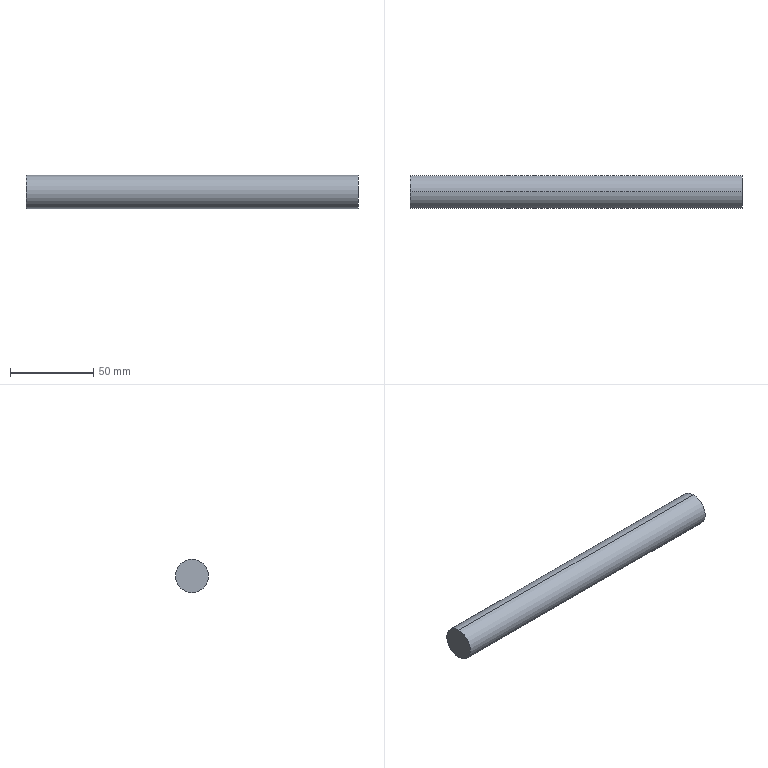Part | STEP file | B1-009 | 1 solid | 8 faces | box 200 x 20 x 20 mm | volume 62632 mm3 | cylinder 4 | cone 2 | plane 2 | commonest cylinder face diameters 4.2 x2 20 x2
STEP:
#1=CARTESIAN_POINT('',(0.,0.,0.));
#2=DIRECTION('',(0.,0.,1.));
#3=DIRECTION('',(1.,0.,0.));
#4=AXIS2_PLACEMENT_3D('',#1,#2,#3);
#5=CARTESIAN_POINT('',(86.,0.,-2.1));
#6=VERTEX_POINT('',#5);
#7=CARTESIAN_POINT('',(100.,0.,-2.1));
#8=VERTEX_POINT('',#7);
#9=CARTESIAN_POINT('',(100.,0.,-2.1));
#10=DIRECTION('',(1.,0.,0.));
#11=VECTOR('',#10,1.);
#12=LINE('',#9,#11);
#13=CARTESIAN_POINT('',(100.,0.,0.));
#14=DIRECTION('',(1.,0.,0.));
#15=DIRECTION('',(0.,0.,-1.));
#16=AXIS2_PLACEMENT_3D('',#13,#14,#15);
#17=CYLINDRICAL_SURFACE('',#16,2.1);
#18=CARTESIAN_POINT('',(6.283,0.));
#19=DIRECTION('',(0.,1.));
#20=VECTOR('',#19,1.);
#21=LINE('',#18,#20);
#22=(GEOMETRIC_REPRESENTATION_CONTEXT(2)PARAMETRIC_REPRESENTATION_CONTEXT()REPRESENTATION_CONTEXT('',''));
#23=DEFINITIONAL_REPRESENTATION('',(#21),#22);
#24=PCURVE('',#17,#23);
#25=CARTESIAN_POINT('',(100.,0.,0.));
#26=DIRECTION('',(1.,0.,0.));
#27=DIRECTION('',(0.,0.,-1.));
#28=AXIS2_PLACEMENT_3D('',#25,#26,#27);
#29=CYLINDRICAL_SURFACE('',#28,2.1);
#30=CARTESIAN_POINT('',(0.,0.));
#31=DIRECTION('',(0.,1.));
#32=VECTOR('',#31,1.);
#33=LINE('',#30,#32);
#34=(GEOMETRIC_REPRESENTATION_CONTEXT(2)PARAMETRIC_REPRESENTATION_CONTEXT()REPRESENTATION_CONTEXT('',''));
#35=DEFINITIONAL_REPRESENTATION('',(#33),#34);
#36=PCURVE('',#29,#35);
#37=SURFACE_CURVE('',#12,(#24,#36),.PCURVE_S1.);
#38=EDGE_CURVE('',#6,#8,#37,.T.);
#39=ORIENTED_EDGE('',*,*,#38,.T.);
#40=CARTESIAN_POINT('',(100.,0.,2.1));
#41=VERTEX_POINT('',#40);
#42=CARTESIAN_POINT('',(100.,0.,0.));
#43=DIRECTION('',(1.,0.,0.));
#44=DIRECTION('',(0.,0.,-1.));
#45=AXIS2_PLACEMENT_3D('',#42,#43,#44);
#46=CIRCLE('',#45,2.1);
#47=CARTESIAN_POINT('',(0.,0.));
#48=DIRECTION('',(1.,0.));
#49=VECTOR('',#48,1.);
#50=LINE('',#47,#49);
#51=(GEOMETRIC_REPRESENTATION_CONTEXT(2)PARAMETRIC_REPRESENTATION_CONTEXT()REPRESENTATION_CONTEXT('',''));
#52=DEFINITIONAL_REPRESENTATION('',(#50),#51);
#53=PCURVE('',#17,#52);
#54=CARTESIAN_POINT('',(100.,0.,0.));
#55=DIRECTION('',(1.,0.,0.));
#56=DIRECTION('',(0.,0.,-1.));
#57=AXIS2_PLACEMENT_3D('',#54,#55,#56);
#58=PLANE('',#57);
#59=CARTESIAN_POINT('',(0.,0.));
#60=DIRECTION('',(1.,0.));
#61=AXIS2_PLACEMENT_2D('',#59,#60);
#62=CIRCLE('',#61,2.1);
#63=(GEOMETRIC_REPRESENTATION_CONTEXT(2)PARAMETRIC_REPRESENTATION_CONTEXT()REPRESENTATION_CONTEXT('',''));
#64=DEFINITIONAL_REPRESENTATION('',(#62),#63);
#65=PCURVE('',#58,#64);
#66=SURFACE_CURVE('',#46,(#53,#65),.PCURVE_S1.);
#67=EDGE_CURVE('',#41,#8,#66,.T.);
#68=ORIENTED_EDGE('',*,*,#67,.F.);
#69=CARTESIAN_POINT('',(86.,0.,2.1));
#70=VERTEX_POINT('',#69);
#71=CARTESIAN_POINT('',(100.,0.,2.1));
#72=DIRECTION('',(1.,0.,0.));
#73=VECTOR('',#72,1.);
#74=LINE('',#71,#73);
#75=CARTESIAN_POINT('',(3.142,0.));
#76=DIRECTION('',(0.,1.));
#77=VECTOR('',#76,1.);
#78=LINE('',#75,#77);
#79=(GEOMETRIC_REPRESENTATION_CONTEXT(2)PARAMETRIC_REPRESENTATION_CONTEXT()REPRESENTATION_CONTEXT('',''));
#80=DEFINITIONAL_REPRESENTATION('',(#78),#79);
#81=PCURVE('',#17,#80);
#82=CARTESIAN_POINT('',(3.142,0.));
#83=DIRECTION('',(0.,1.));
#84=VECTOR('',#83,1.);
#85=LINE('',#82,#84);
#86=(GEOMETRIC_REPRESENTATION_CONTEXT(2)PARAMETRIC_REPRESENTATION_CONTEXT()REPRESENTATION_CONTEXT('',''));
#87=DEFINITIONAL_REPRESENTATION('',(#85),#86);
#88=PCURVE('',#29,#87);
#89=SURFACE_CURVE('',#74,(#81,#88),.PCURVE_S1.);
#90=EDGE_CURVE('',#70,#41,#89,.T.);
#91=ORIENTED_EDGE('',*,*,#90,.F.);
#92=CARTESIAN_POINT('',(86.,0.,0.));
#93=DIRECTION('',(1.,0.,0.));
#94=DIRECTION('',(0.,0.,-1.));
#95=AXIS2_PLACEMENT_3D('',#92,#93,#94);
#96=CIRCLE('',#95,2.1);
#97=CARTESIAN_POINT('',(0.,-14.));
#98=DIRECTION('',(1.,0.));
#99=VECTOR('',#98,1.);
#100=LINE('',#97,#99);
#101=(GEOMETRIC_REPRESENTATION_CONTEXT(2)PARAMETRIC_REPRESENTATION_CONTEXT()REPRESENTATION_CONTEXT('',''));
#102=DEFINITIONAL_REPRESENTATION('',(#100),#101);
#103=PCURVE('',#17,#102);
#104=CARTESIAN_POINT('',(86.,0.,0.));
#105=DIRECTION('',(1.,0.,0.));
#106=DIRECTION('',(0.,0.,-1.));
#107=AXIS2_PLACEMENT_3D('',#104,#105,#106);
#108=CONICAL_SURFACE('',#107,2.1,1.03);
#109=CARTESIAN_POINT('',(0.,0.));
#110=DIRECTION('',(1.,0.));
#111=VECTOR('',#110,1.);
#112=LINE('',#109,#111);
#113=(GEOMETRIC_REPRESENTATION_CONTEXT(2)PARAMETRIC_REPRESENTATION_CONTEXT()REPRESENTATION_CONTEXT('',''));
#114=DEFINITIONAL_REPRESENTATION('',(#112),#113);
#115=PCURVE('',#108,#114);
#116=SURFACE_CURVE('',#96,(#103,#115),.PCURVE_S1.);
#117=EDGE_CURVE('',#70,#6,#116,.T.);
#118=ORIENTED_EDGE('',*,*,#117,.T.);
#119=EDGE_LOOP('',(#39,#68,#91,#118));
#120=FACE_BOUND('',#119,.F.);
#121=ADVANCED_FACE('',(#120),#17,.F.);
#122=ORIENTED_EDGE('',*,*,#117,.F.);
#123=CARTESIAN_POINT('',(84.738,0.,0.));
#124=VERTEX_POINT('',#123);
#125=CARTESIAN_POINT('',(86.,0.,2.1));
#126=DIRECTION('',(0.515,0.,0.8572));
#127=VECTOR('',#126,1.);
#128=LINE('',#125,#127);
#129=CARTESIAN_POINT('',(3.142,0.));
#130=DIRECTION('',(0.,1.));
#131=VECTOR('',#130,1.);
#132=LINE('',#129,#131);
#133=(GEOMETRIC_REPRESENTATION_CONTEXT(2)PARAMETRIC_REPRESENTATION_CONTEXT()REPRESENTATION_CONTEXT('',''));
#134=DEFINITIONAL_REPRESENTATION('',(#132),#133);
#135=PCURVE('',#108,#134);
#136=CARTESIAN_POINT('',(86.,0.,0.));
#137=DIRECTION('',(1.,0.,0.));
#138=DIRECTION('',(0.,0.,-1.));
#139=AXIS2_PLACEMENT_3D('',#136,#137,#138);
#140=CONICAL_SURFACE('',#139,2.1,1.03);
#141=CARTESIAN_POINT('',(3.142,0.));
#142=DIRECTION('',(0.,1.));
#143=VECTOR('',#142,1.);
#144=LINE('',#141,#143);
#145=(GEOMETRIC_REPRESENTATION_CONTEXT(2)PARAMETRIC_REPRESENTATION_CONTEXT()REPRESENTATION_CONTEXT('',''));
#146=DEFINITIONAL_REPRESENTATION('',(#144),#145);
#147=PCURVE('',#140,#146);
#148=SURFACE_CURVE('',#128,(#135,#147),.PCURVE_S1.);
#149=EDGE_CURVE('',#124,#70,#148,.T.);
#150=ORIENTED_EDGE('',*,*,#149,.F.);
#151=CARTESIAN_POINT('',(86.,0.,-2.1));
#152=DIRECTION('',(0.515,0.,-0.8572));
#153=VECTOR('',#152,1.);
#154=LINE('',#151,#153);
#155=CARTESIAN_POINT('',(6.283,0.));
#156=DIRECTION('',(0.,1.));
#157=VECTOR('',#156,1.);
#158=LINE('',#155,#157);
#159=(GEOMETRIC_REPRESENTATION_CONTEXT(2)PARAMETRIC_REPRESENTATION_CONTEXT()REPRESENTATION_CONTEXT('',''));
#160=DEFINITIONAL_REPRESENTATION('',(#158),#159);
#161=PCURVE('',#108,#160);
#162=CARTESIAN_POINT('',(0.,0.));
#163=DIRECTION('',(0.,1.));
#164=VECTOR('',#163,1.);
#165=LINE('',#162,#164);
#166=(GEOMETRIC_REPRESENTATION_CONTEXT(2)PARAMETRIC_REPRESENTATION_CONTEXT()REPRESENTATION_CONTEXT('',''));
#167=DEFINITIONAL_REPRESENTATION('',(#165),#166);
#168=PCURVE('',#140,#167);
#169=SURFACE_CURVE('',#154,(#161,#168),.PCURVE_S1.);
#170=EDGE_CURVE('',#124,#6,#169,.T.);
#171=ORIENTED_EDGE('',*,*,#170,.T.);
#172=EDGE_LOOP('',(#122,#150,#171));
#173=FACE_BOUND('',#172,.F.);
#174=ADVANCED_FACE('',(#173),#108,.F.);
#175=CARTESIAN_POINT('',(100.,0.,-10.));
#176=VERTEX_POINT('',#175);
#177=CARTESIAN_POINT('',(100.,0.,10.));
#178=VERTEX_POINT('',#177);
#179=CARTESIAN_POINT('',(100.,0.,0.));
#180=DIRECTION('',(1.,0.,0.));
#181=DIRECTION('',(0.,0.,-1.));
#182=AXIS2_PLACEMENT_3D('',#179,#180,#181);
#183=CIRCLE('',#182,10.);
#184=CARTESIAN_POINT('',(100.,0.,0.));
#185=DIRECTION('',(-1.,0.,0.));
#186=DIRECTION('',(0.,0.,1.));
#187=AXIS2_PLACEMENT_3D('',#184,#185,#186);
#188=CYLINDRICAL_SURFACE('',#187,10.);
#189=CARTESIAN_POINT('',(3.142,0.));
#190=DIRECTION('',(-1.,0.));
#191=VECTOR('',#190,1.);
#192=LINE('',#189,#191);
#193=(GEOMETRIC_REPRESENTATION_CONTEXT(2)PARAMETRIC_REPRESENTATION_CONTEXT()REPRESENTATION_CONTEXT('',''));
#194=DEFINITIONAL_REPRESENTATION('',(#192),#193);
#195=PCURVE('',#188,#194);
#196=CARTESIAN_POINT('',(0.,0.));
#197=DIRECTION('',(1.,0.));
#198=AXIS2_PLACEMENT_2D('',#196,#197);
#199=CIRCLE('',#198,10.);
#200=(GEOMETRIC_REPRESENTATION_CONTEXT(2)PARAMETRIC_REPRESENTATION_CONTEXT()REPRESENTATION_CONTEXT('',''));
#201=DEFINITIONAL_REPRESENTATION('',(#199),#200);
#202=PCURVE('',#58,#201);
#203=SURFACE_CURVE('',#183,(#195,#202),.PCURVE_S1.);
#204=EDGE_CURVE('',#176,#178,#203,.T.);
#205=ORIENTED_EDGE('',*,*,#204,.F.);
#206=CARTESIAN_POINT('',(-100.,0.,-10.));
#207=VERTEX_POINT('',#206);
#208=CARTESIAN_POINT('',(100.,0.,-10.));
#209=DIRECTION('',(-1.,0.,0.));
#210=VECTOR('',#209,1.);
#211=LINE('',#208,#210);
#212=CARTESIAN_POINT('',(3.142,0.));
#213=DIRECTION('',(0.,1.));
#214=VECTOR('',#213,1.);
#215=LINE('',#212,#214);
#216=(GEOMETRIC_REPRESENTATION_CONTEXT(2)PARAMETRIC_REPRESENTATION_CONTEXT()REPRESENTATION_CONTEXT('',''));
#217=DEFINITIONAL_REPRESENTATION('',(#215),#216);
#218=PCURVE('',#188,#217);
#219=CARTESIAN_POINT('',(100.,0.,0.));
#220=DIRECTION('',(-1.,0.,0.));
#221=DIRECTION('',(0.,0.,1.));
#222=AXIS2_PLACEMENT_3D('',#219,#220,#221);
#223=CYLINDRICAL_SURFACE('',#222,10.);
#224=CARTESIAN_POINT('',(3.142,0.));
#225=DIRECTION('',(0.,1.));
#226=VECTOR('',#225,1.);
#227=LINE('',#224,#226);
#228=(GEOMETRIC_REPRESENTATION_CONTEXT(2)PARAMETRIC_REPRESENTATION_CONTEXT()REPRESENTATION_CONTEXT('',''));
#229=DEFINITIONAL_REPRESENTATION('',(#227),#228);
#230=PCURVE('',#223,#229);
#231=SURFACE_CURVE('',#211,(#218,#230),.PCURVE_S1.);
#232=EDGE_CURVE('',#176,#207,#231,.T.);
#233=ORIENTED_EDGE('',*,*,#232,.T.);
#234=CARTESIAN_POINT('',(-100.,0.,10.));
#235=VERTEX_POINT('',#234);
#236=CARTESIAN_POINT('',(-100.,0.,0.));
#237=DIRECTION('',(1.,0.,0.));
#238=DIRECTION('',(0.,0.,-1.));
#239=AXIS2_PLACEMENT_3D('',#236,#237,#238);
#240=CIRCLE('',#239,10.);
#241=CARTESIAN_POINT('',(3.142,200.));
#242=DIRECTION('',(-1.,0.));
#243=VECTOR('',#242,1.);
#244=LINE('',#241,#243);
#245=(GEOMETRIC_REPRESENTATION_CONTEXT(2)PARAMETRIC_REPRESENTATION_CONTEXT()REPRESENTATION_CONTEXT('',''));
#246=DEFINITIONAL_REPRESENTATION('',(#244),#245);
#247=PCURVE('',#188,#246);
#248=CARTESIAN_POINT('',(-100.,0.,0.));
#249=DIRECTION('',(1.,0.,0.));
#250=DIRECTION('',(0.,0.,-1.));
#251=AXIS2_PLACEMENT_3D('',#248,#249,#250);
#252=PLANE('',#251);
#253=CARTESIAN_POINT('',(0.,0.));
#254=DIRECTION('',(1.,0.));
#255=AXIS2_PLACEMENT_2D('',#253,#254);
#256=CIRCLE('',#255,10.);
#257=(GEOMETRIC_REPRESENTATION_CONTEXT(2)PARAMETRIC_REPRESENTATION_CONTEXT()REPRESENTATION_CONTEXT('',''));
#258=DEFINITIONAL_REPRESENTATION('',(#256),#257);
#259=PCURVE('',#252,#258);
#260=SURFACE_CURVE('',#240,(#247,#259),.PCURVE_S1.);
#261=EDGE_CURVE('',#207,#235,#260,.T.);
#262=ORIENTED_EDGE('',*,*,#261,.T.);
#263=CARTESIAN_POINT('',(100.,0.,10.));
#264=DIRECTION('',(-1.,0.,0.));
#265=VECTOR('',#264,1.);
#266=LINE('',#263,#265);
#267=CARTESIAN_POINT('',(0.,0.));
#268=DIRECTION('',(0.,1.));
#269=VECTOR('',#268,1.);
#270=LINE('',#267,#269);
#271=(GEOMETRIC_REPRESENTATION_CONTEXT(2)PARAMETRIC_REPRESENTATION_CONTEXT()REPRESENTATION_CONTEXT('',''));
#272=DEFINITIONAL_REPRESENTATION('',(#270),#271);
#273=PCURVE('',#188,#272);
#274=CARTESIAN_POINT('',(6.283,0.));
#275=DIRECTION('',(0.,1.));
#276=VECTOR('',#275,1.);
#277=LINE('',#274,#276);
#278=(GEOMETRIC_REPRESENTATION_CONTEXT(2)PARAMETRIC_REPRESENTATION_CONTEXT()REPRESENTATION_CONTEXT('',''));
#279=DEFINITIONAL_REPRESENTATION('',(#277),#278);
#280=PCURVE('',#223,#279);
#281=SURFACE_CURVE('',#266,(#273,#280),.PCURVE_S1.);
#282=EDGE_CURVE('',#178,#235,#281,.T.);
#283=ORIENTED_EDGE('',*,*,#282,.F.);
#284=EDGE_LOOP('',(#205,#233,#262,#283));
#285=FACE_BOUND('',#284,.T.);
#286=ADVANCED_FACE('',(#285),#188,.T.);
#287=ORIENTED_EDGE('',*,*,#232,.F.);
#288=CARTESIAN_POINT('',(100.,0.,0.));
#289=DIRECTION('',(1.,0.,0.));
#290=DIRECTION('',(0.,0.,-1.));
#291=AXIS2_PLACEMENT_3D('',#288,#289,#290);
#292=CIRCLE('',#291,10.);
#293=CARTESIAN_POINT('',(9.425,0.));
#294=DIRECTION('',(-1.,0.));
#295=VECTOR('',#294,1.);
#296=LINE('',#293,#295);
#297=(GEOMETRIC_REPRESENTATION_CONTEXT(2)PARAMETRIC_REPRESENTATION_CONTEXT()REPRESENTATION_CONTEXT('',''));
#298=DEFINITIONAL_REPRESENTATION('',(#296),#297);
#299=PCURVE('',#223,#298);
#300=CARTESIAN_POINT('',(0.,0.));
#301=DIRECTION('',(1.,0.));
#302=AXIS2_PLACEMENT_2D('',#300,#301);
#303=CIRCLE('',#302,10.);
#304=(GEOMETRIC_REPRESENTATION_CONTEXT(2)PARAMETRIC_REPRESENTATION_CONTEXT()REPRESENTATION_CONTEXT('',''));
#305=DEFINITIONAL_REPRESENTATION('',(#303),#304);
#306=PCURVE('',#58,#305);
#307=SURFACE_CURVE('',#292,(#299,#306),.PCURVE_S1.);
#308=EDGE_CURVE('',#178,#176,#307,.T.);
#309=ORIENTED_EDGE('',*,*,#308,.F.);
#310=ORIENTED_EDGE('',*,*,#282,.T.);
#311=CARTESIAN_POINT('',(-100.,0.,0.));
#312=DIRECTION('',(1.,0.,0.));
#313=DIRECTION('',(0.,0.,-1.));
#314=AXIS2_PLACEMENT_3D('',#311,#312,#313);
#315=CIRCLE('',#314,10.);
#316=CARTESIAN_POINT('',(9.425,200.));
#317=DIRECTION('',(-1.,0.));
#318=VECTOR('',#317,1.);
#319=LINE('',#316,#318);
#320=(GEOMETRIC_REPRESENTATION_CONTEXT(2)PARAMETRIC_REPRESENTATION_CONTEXT()REPRESENTATION_CONTEXT('',''));
#321=DEFINITIONAL_REPRESENTATION('',(#319),#320);
#322=PCURVE('',#223,#321);
#323=CARTESIAN_POINT('',(0.,0.));
#324=DIRECTION('',(1.,0.));
#325=AXIS2_PLACEMENT_2D('',#323,#324);
#326=CIRCLE('',#325,10.);
#327=(GEOMETRIC_REPRESENTATION_CONTEXT(2)PARAMETRIC_REPRESENTATION_CONTEXT()REPRESENTATION_CONTEXT('',''));
#328=DEFINITIONAL_REPRESENTATION('',(#326),#327);
#329=PCURVE('',#252,#328);
#330=SURFACE_CURVE('',#315,(#322,#329),.PCURVE_S1.);
#331=EDGE_CURVE('',#235,#207,#330,.T.);
#332=ORIENTED_EDGE('',*,*,#331,.T.);
#333=EDGE_LOOP('',(#287,#309,#310,#332));
#334=FACE_BOUND('',#333,.T.);
#335=ADVANCED_FACE('',(#334),#223,.T.);
#336=CARTESIAN_POINT('',(100.,0.,0.));
#337=DIRECTION('',(1.,0.,0.));
#338=DIRECTION('',(0.,0.,-1.));
#339=AXIS2_PLACEMENT_3D('',#336,#337,#338);
#340=CIRCLE('',#339,2.1);
#341=CARTESIAN_POINT('',(0.,0.));
#342=DIRECTION('',(1.,0.));
#343=AXIS2_PLACEMENT_2D('',#341,#342);
#344=CIRCLE('',#343,2.1);
#345=(GEOMETRIC_REPRESENTATION_CONTEXT(2)PARAMETRIC_REPRESENTATION_CONTEXT()REPRESENTATION_CONTEXT('',''));
#346=DEFINITIONAL_REPRESENTATION('',(#344),#345);
#347=PCURVE('',#58,#346);
#348=CARTESIAN_POINT('',(0.,0.));
#349=DIRECTION('',(1.,0.));
#350=VECTOR('',#349,1.);
#351=LINE('',#348,#350);
#352=(GEOMETRIC_REPRESENTATION_CONTEXT(2)PARAMETRIC_REPRESENTATION_CONTEXT()REPRESENTATION_CONTEXT('',''));
#353=DEFINITIONAL_REPRESENTATION('',(#351),#352);
#354=PCURVE('',#29,#353);
#355=SURFACE_CURVE('',#340,(#347,#354),.PCURVE_S1.);
#356=EDGE_CURVE('',#8,#41,#355,.T.);
#357=ORIENTED_EDGE('',*,*,#356,.F.);
#358=ORIENTED_EDGE('',*,*,#67,.F.);
#359=EDGE_LOOP('',(#357,#358));
#360=FACE_BOUND('',#359,.T.);
#361=ORIENTED_EDGE('',*,*,#308,.T.);
#362=ORIENTED_EDGE('',*,*,#204,.T.);
#363=EDGE_LOOP('',(#361,#362));
#364=FACE_BOUND('',#363,.T.);
#365=ADVANCED_FACE('',(#360,#364),#58,.T.);
#366=ORIENTED_EDGE('',*,*,#331,.F.);
#367=ORIENTED_EDGE('',*,*,#261,.F.);
#368=EDGE_LOOP('',(#366,#367));
#369=FACE_BOUND('',#368,.T.);
#370=ADVANCED_FACE('',(#369),#252,.F.);
#371=CARTESIAN_POINT('',(86.,0.,0.));
#372=DIRECTION('',(1.,0.,0.));
#373=DIRECTION('',(0.,0.,-1.));
#374=AXIS2_PLACEMENT_3D('',#371,#372,#373);
#375=CIRCLE('',#374,2.1);
#376=CARTESIAN_POINT('',(0.,0.));
#377=DIRECTION('',(1.,0.));
#378=VECTOR('',#377,1.);
#379=LINE('',#376,#378);
#380=(GEOMETRIC_REPRESENTATION_CONTEXT(2)PARAMETRIC_REPRESENTATION_CONTEXT()REPRESENTATION_CONTEXT('',''));
#381=DEFINITIONAL_REPRESENTATION('',(#379),#380);
#382=PCURVE('',#140,#381);
#383=CARTESIAN_POINT('',(0.,-14.));
#384=DIRECTION('',(1.,0.));
#385=VECTOR('',#384,1.);
#386=LINE('',#383,#385);
#387=(GEOMETRIC_REPRESENTATION_CONTEXT(2)PARAMETRIC_REPRESENTATION_CONTEXT()REPRESENTATION_CONTEXT('',''));
#388=DEFINITIONAL_REPRESENTATION('',(#386),#387);
#389=PCURVE('',#29,#388);
#390=SURFACE_CURVE('',#375,(#382,#389),.PCURVE_S1.);
#391=EDGE_CURVE('',#6,#70,#390,.T.);
#392=ORIENTED_EDGE('',*,*,#391,.F.);
#393=ORIENTED_EDGE('',*,*,#170,.F.);
#394=ORIENTED_EDGE('',*,*,#149,.T.);
#395=EDGE_LOOP('',(#392,#393,#394));
#396=FACE_BOUND('',#395,.F.);
#397=ADVANCED_FACE('',(#396),#140,.F.);
#398=ORIENTED_EDGE('',*,*,#356,.F.);
#399=ORIENTED_EDGE('',*,*,#38,.F.);
#400=ORIENTED_EDGE('',*,*,#391,.T.);
#401=ORIENTED_EDGE('',*,*,#90,.T.);
#402=EDGE_LOOP('',(#398,#399,#400,#401));
#403=FACE_BOUND('',#402,.F.);
#404=ADVANCED_FACE('',(#403),#29,.F.);
#405=CLOSED_SHELL('',(#121,#174,#286,#335,#365,#370,#397,#404));
#406=MANIFOLD_SOLID_BREP('',#405);
#407=(LENGTH_UNIT()NAMED_UNIT(*)SI_UNIT(.MILLI.,.METRE.));
#408=UNCERTAINTY_MEASURE_WITH_UNIT(LENGTH_MEASURE(0.0000001),#407,'','');
#409=(NAMED_UNIT(*)PLANE_ANGLE_UNIT()SI_UNIT($,.RADIAN.));
#410=(NAMED_UNIT(*)SI_UNIT($,.STERADIAN.)SOLID_ANGLE_UNIT());
#411=(GEOMETRIC_REPRESENTATION_CONTEXT(3)GLOBAL_UNCERTAINTY_ASSIGNED_CONTEXT((#408))GLOBAL_UNIT_ASSIGNED_CONTEXT((#407,#409,#410))REPRESENTATION_CONTEXT('',''));
#412=ADVANCED_BREP_SHAPE_REPRESENTATION('',(#4,#406),#411);